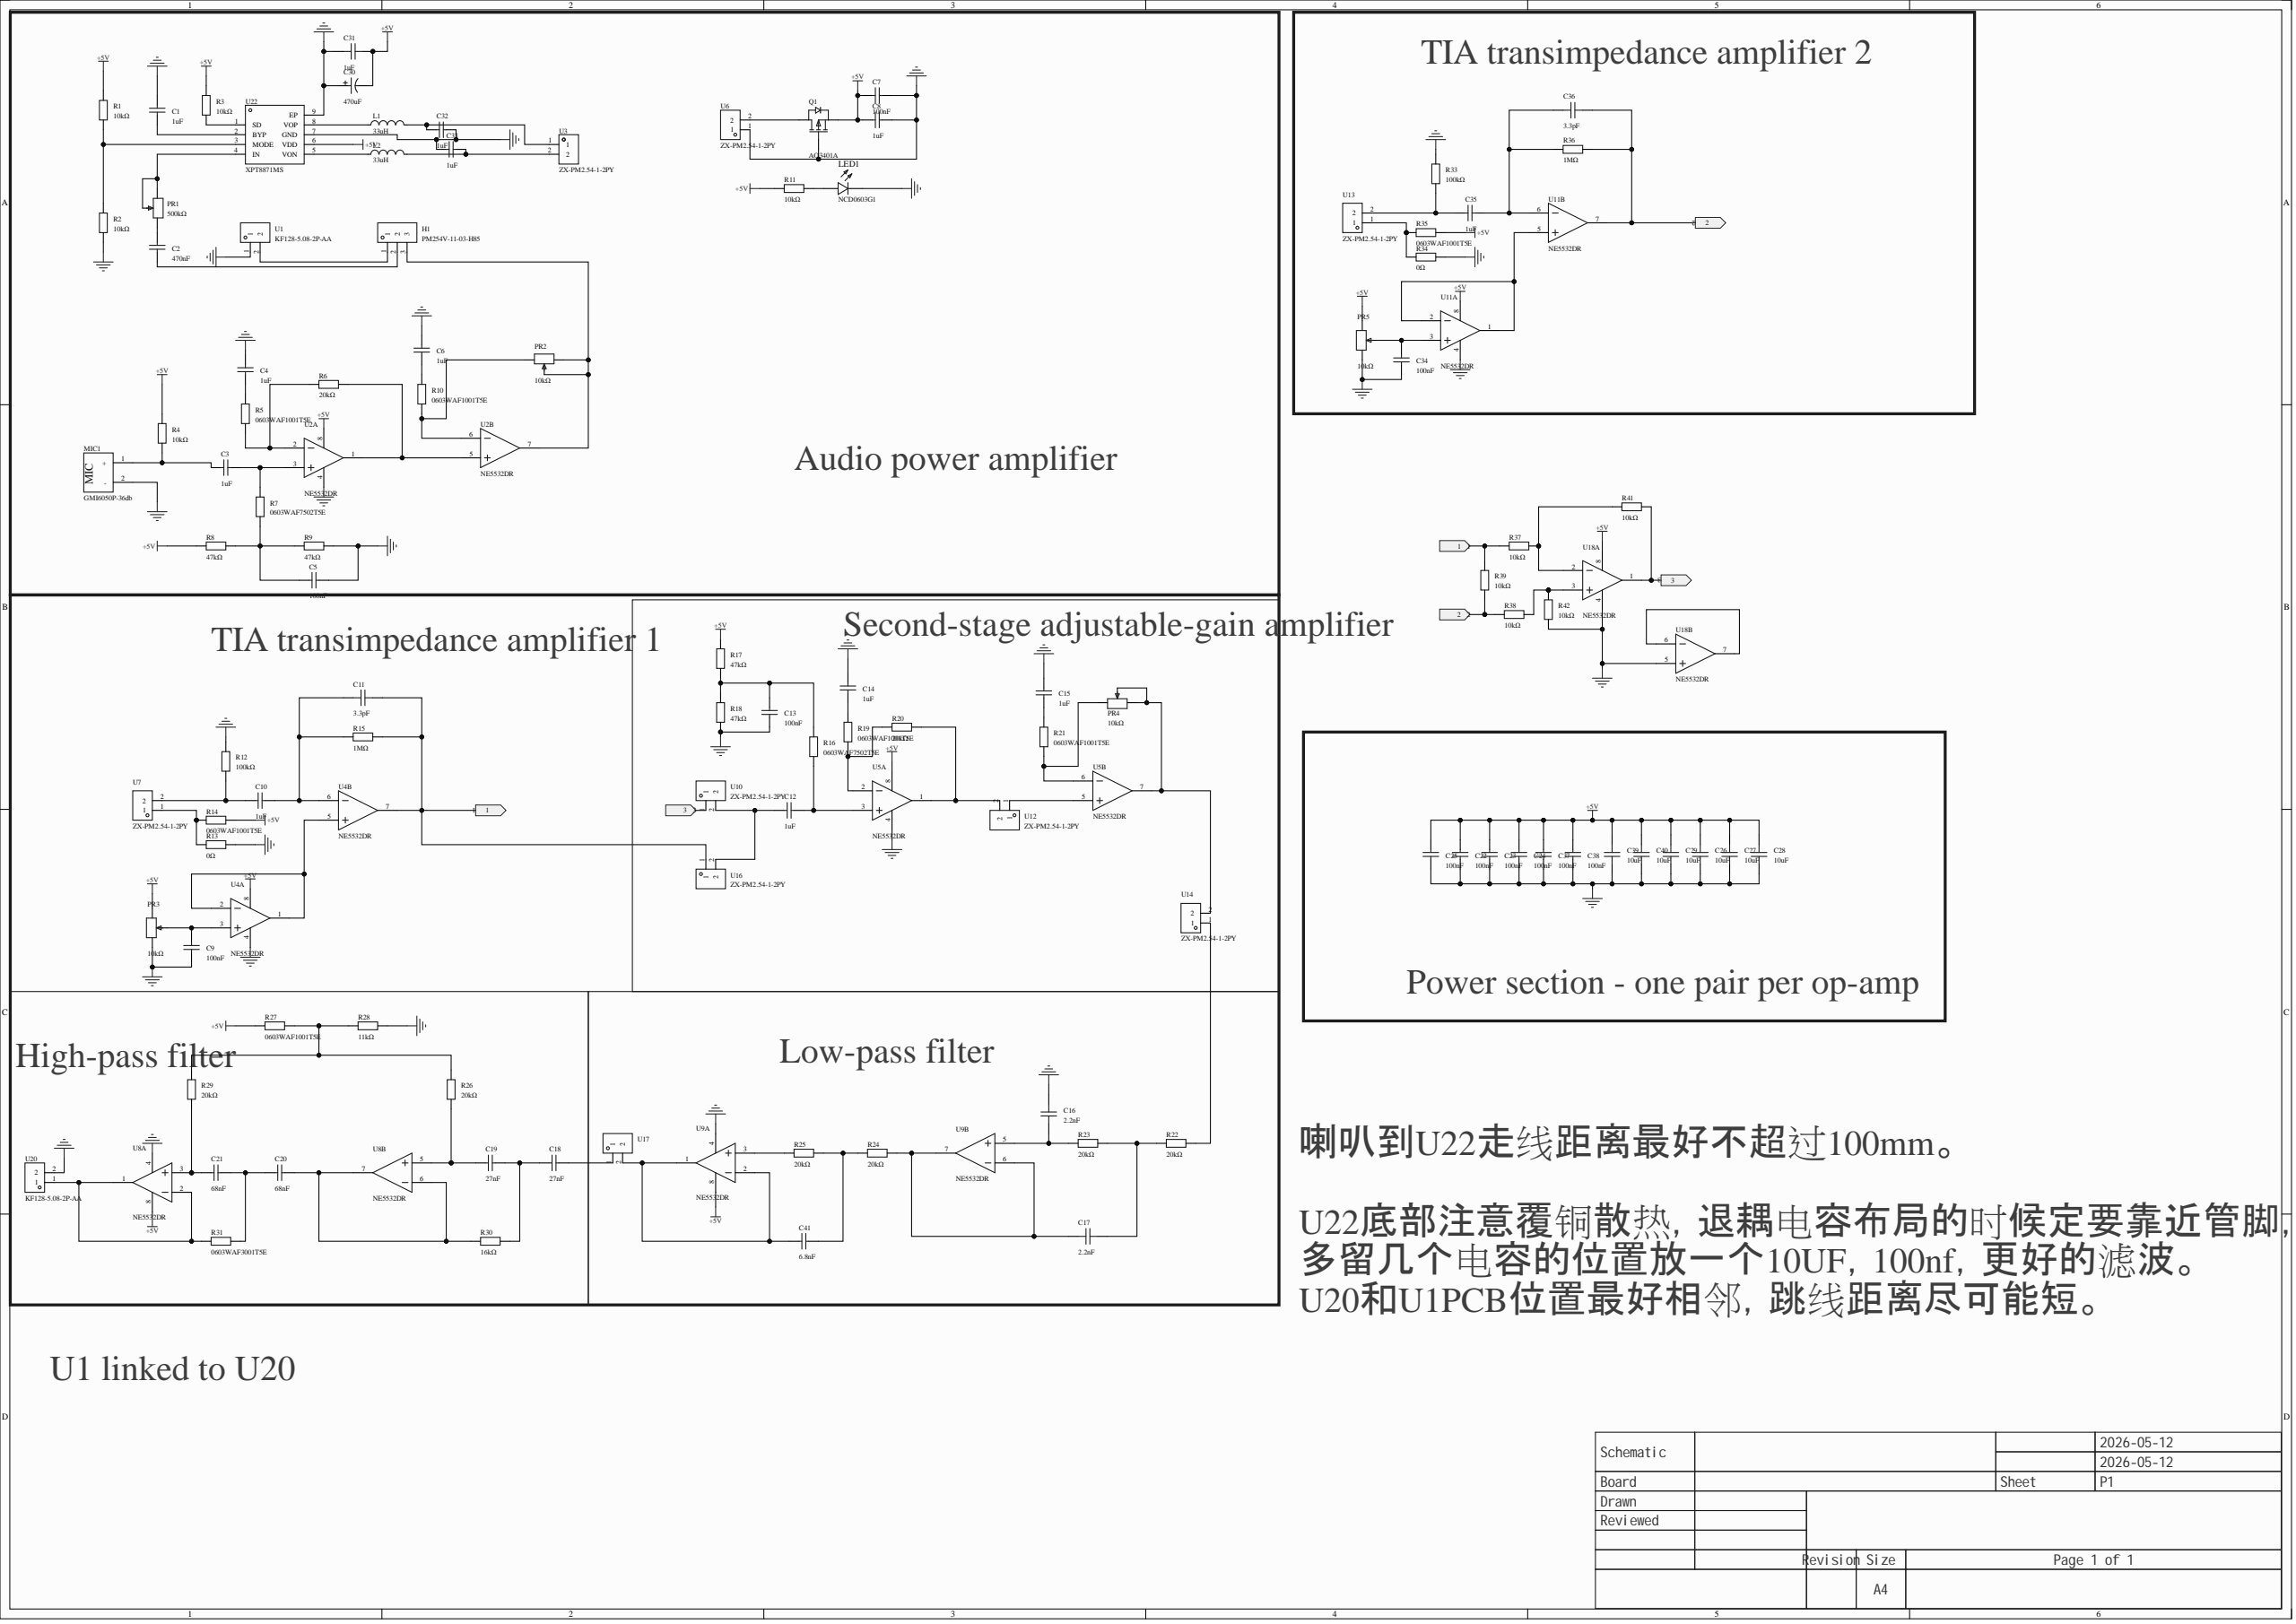Circuit board | Altium Designer | 111 parts | 65 nets
Bill of materials:
Comment,Description,Designator,Footprint,LibRef,Quantity
"1uF","Temperature coefficient: X5R; Tolerance: ±10%; Rated voltage: 50V; Capacitance: 1uF;, Capacitance: 1uF; Tolerance: ±10%; Rated voltage: 50V; Temperature coefficient: X5R;","C1, C3, C4, C6, C8, C10, C12, C14, C15, C31, C32, C33, C35","C0603","CL10A105KB8NNNC","13"
"470nF","Capacitance: 470nF; Tolerance: ±10%; Rated voltage: 16V; Dielectric (temp. coefficient): X7R;","C2","C0603","CC0603KRX7R7BB474","1"
"100nF","Capacitance: 100nF; Tolerance: ±10%; Rated voltage: 100V; Dielectric (temp. coefficient): X7R;","C5, C7, C9, C13, C22, C23, C24, C25, C34, C37, C38","C0805","CC0805KKX7R0BB104","11"
"3.3pF","Capacitance: 3.3pF; Tolerance: ±0.1pF; Rated voltage: 50V; Dielectric (temp. coefficient): NP0;","C11, C36","C0402","CC0402BRNPO9BN3R3","2"
"2.2nF","Temperature coefficient: X7R; Capacitance: 2.2nF; Tolerance: ±10%; Rated voltage: 50V;","C16, C17","C0805","TCC0805X7R222K500DTS","2"
"27nF","Capacitance: 27nF; Tolerance: ±10%; Rated voltage: 50V; Dielectric (temp. coefficient): X7R;","C18, C19","C0603","CC0603KRX7R9BB273","2"
"68nF","Temperature coefficient: X7R; Tolerance: ±10%; Capacitance: 68nF; Rated voltage: 50V;","C20, C21","C0603","CL10B683KB8NNNC","2"
"10uF","Capacitance: 10uF; Tolerance: ±20%; Rated voltage: 25V; Temperature coefficient: X5R;","C26, C27, C28, C29, C39, C40","C0603","CL10A106MA8NRNC","6"
"470uF","Capacitance: 470uF; Tolerance: ±20%; Rated voltage: 35V;","C30","CAP-TH_BD10.0-P5.00-D1.0-FD","35YXJ470M10x16","1"
"6.8nF","Capacitance: 6.8nF; Tolerance: ±10%; Rated voltage: 50V; Dielectric (temp. coefficient): X7R;","C41","C0603","CC0603KRX7R9BB682","1"
"PM254V-11-03-H85","Socket structure: 1x3P; Pitch: 2.54mm; Row spacing: -; Round/square hole: Square; Mounting type: Through-hole; Rows: Single row; Total positions: 3P; Rated current: 3A; Socket orientation: Top; Plastic height: 8.5mm; Contact material: Brass; Contact plating: -; Operating temperature: -40℃~+105℃;","H1","HDR-TH_3P-P2.54-V-F","PM254V-11-03-H85","1"
"33uH","Inductance: 33uH; Tolerance: ±20%; Rated current: 2A; DC resistance (DCR): 270mΩ;","L1, L2","IND-SMD_L7.3-W6.6","MHCI06030-330M-R8","2"
"NCD0603G1","Emitted color: Emerald green;","LED1","LED0603-RD","NCD0603G1","1"
"GMI6050P-36db","","MIC1","MIC-TH_BD6.0-P1.90-D0.4-L-FD_GMI6050P-2CXXDB","GMI6050P-36db","1"
"500kΩ","Resistance: 500kΩ; Tolerance: ±10%; Temperature coefficient: ±100ppm/?;","PR1","RES-ADJ-TH_3296W","3296W-1-504LF","1"
"10kΩ","Resistance: 10kΩ; Tolerance: ±10%; Temperature coefficient: ±100ppm/?;","PR2, PR3, PR4, PR5","RES-ADJ-TH_3296W","3296W-1-103LF","4"
"AO3401A","","Q1","SOT-23_L2.9-W1.3-P1.90-LS2.4-BR","AO3401A_C15127","1"
"10kΩ","","R1, R2, R3, R4, R11, R37, R38, R39, R41, R42","R0603","0603WAF1002T5E","10"
"0603WAF1001T5E","","R5, R10, R14, R19, R21, R27, R35","R0603","0603WAF1001T5E","7"
"20kΩ","","R6, R20, R22, R23, R24, R25, R26, R29","R0603","0603WAF2002T5E","8"
"0603WAF7502T5E","","R7, R16","R0603","0603WAF7502T5E","2"
"47kΩ","","R8, R9, R17, R18","R0603","0603WAF4702T5E","4"
"100kΩ","","R12, R33","R0603","0603WAF1003T5E","2"
"0Ω","","R13, R34","R0603","0603WAF0000T5E","2"
"1MΩ","","R15, R36","R0603","0603WAF1004T5E","2"
"11kΩ","","R28","R0603","0603WAF1102T5E","1"
"16kΩ","","R30","R0603","0603WAF1602T5E","1"
"0603WAF3001T5E","","R31","R0603","0603WAF3001T5E","1"
"KF128-5.08-2P-AA","Structure: 1x2P; Pitch: 5.08mm; Color: Green; Mounting type: Through-hole; Rows: 1; Pins per row: 2; Rated current: 24A; Rated voltage: 250V; Wire gauge - AWG: 12~22; Wire gauge - sq mm: 2.5; Operating temperature: -40℃~+105℃;","U1, U20","CONN-TH_P5.08_KF128-5.08-2P","KF128-5.08-2P-AA","2"
"NE5532DR","Op-amp type: General Purpose; Amplifiers per package: 2; Gain bandwidth product (GBP): 10MHz; Slew rate (SR): 9 V/us; Supply voltage: ±5V ~ 15V; Supply current per channel: 8mA;","U2, U4, U5, U8, U9, U11, U18","SOIC-8_L4.9-W3.9-P1.27-LS6.0-BL","NE5532DR","7"
"ZX-PM2.54-1-2PY","Socket structure: 1x2P; Pitch: 2.54mm; Row spacing: -; Round/square hole: Square; Mounting type: Through-hole; Rows: Single row; Total positions: 2P; Rated current: 3A; Rated voltage: -; Socket orientation: Top; Plastic height: 8.5mm; Contact material: Brass; Contact plating: Gold; Operating temperature: -40℃~+105℃;","U3, U6, U7, U10, U12, U13, U14, U16, U17","HDR-TH_2P-P2.54-V-F","ZX-PM2.54-1-2PY","9"
"XPT8871MS","","U22","ESOP-8_L4.9-W3.9-P1.27-LS6.0-BL-EP","XPT8871MS","1"
Netlist (Protel format):
[
C1
C0603
1uF



]
[
C2
C0603
470nF



]
[
C3
C0603
1uF



]
[
C4
C0603
1uF



]
[
C5
C0805
100nF



]
[
C6
C0603
1uF



]
[
C7
C0805
100nF



]
[
C8
C0603
1uF



]
[
C9
C0805
100nF



]
[
C10
C0603
1uF



]
[
C11
C0402
3.3pF



]
[
C12
C0603
1uF



]
[
C13
C0805
100nF



]
[
C14
C0603
1uF



]
[
C15
C0603
1uF



]
[
C16
C0805
2.2nF



]
[
C17
C0805
2.2nF



]
[
C18
C0603
27nF



]
[
C19
C0603
27nF



]
[
C20
C0603
68nF



]
[
C21
C0603
68nF



]
[
C22
C0805
100nF



]
[
C23
C0805
100nF



]
[
C24
C0805
100nF



]
[
C25
C0805
100nF



]
[
C26
C0603
10uF



]
[
C27
C0603
10uF



]
[
C28
C0603
10uF



]
[
C29
C0603
10uF



]
[
C30
CAP-TH_BD10.0-P5.00-D1.0-FD
470uF



]
[
C31
C0603
1uF



]
[
C32
C0603
1uF



]
[
C33
C0603
1uF



]
[
C34
C0805
100nF



]
[
C35
C0603
1uF



]
[
C36
C0402
3.3pF



]
[
C37
C0805
100nF



]
[
C38
C0805
100nF



]
[
C39
C0603
10uF



]
[
C40
C0603
10uF



]
[
C41
C0603
6.8nF



]
[
H1
HDR-TH_3P-P2.54-V-F
PM254V-11-03-H85



]
[
L1
IND-SMD_L7.3-W6.6
33uH



]
[
L2
IND-SMD_L7.3-W6.6
33uH



]
[
LED1
LED0603-RD
NCD0603G1



]
[
MIC1
MIC-TH_BD6.0-P1.90-D0.4-L-FD_GMI6050P-2CXXDB
GMI6050P-36db



]
[
PR1
RES-ADJ-TH_3296W
500kΩ



]
[
PR2
RES-ADJ-TH_3296W
10kΩ



]
[
PR3
RES-ADJ-TH_3296W
10kΩ



]
[
PR4
RES-ADJ-TH_3296W
10kΩ



]
[
PR5
RES-ADJ-TH_3296W
10kΩ



]
[
Q1
SOT-23_L2.9-W1.3-P1.90-LS2.4-BR
AO3401A



]
[
R1
R0603
10kΩ



]
[
R2
R0603
10kΩ



]
[
R3
R0603
10kΩ



]
[
R4
R0603
10kΩ



]
[
R5
R0603
0603WAF1001T5E



]
[
R6
R0603
20kΩ



]
[
R7
R0603
0603WAF7502T5E



]
[
R8
R0603
47kΩ



]
[
R9
R0603
47kΩ



]
[
R10
R0603
0603WAF1001T5E



]
[
R11
R0603
10kΩ



]
[
R12
R0603
100kΩ



]
[
R13
R0603
0Ω



]
[
R14
R0603
0603WAF1001T5E



]
[
R15
R0603
1MΩ



]
[
R16
R0603
0603WAF7502T5E



]
[
R17
R0603
47kΩ



]
[
R18
R0603
47kΩ



]
[
R19
R0603
0603WAF1001T5E



]
[
R20
R0603
20kΩ



]
[
R21
R0603
0603WAF1001T5E



]
[
R22
R0603
20kΩ



]
[
R23
R0603
20kΩ



]
[
R24
R0603
20kΩ



]
[
R25
R0603
20kΩ



]
[
R26
R0603
20kΩ



]
[
R27
R0603
0603WAF1001T5E



]
[
R28
R0603
11kΩ



]
[
R29
R0603
20kΩ



]
[
R30
R0603
16kΩ



]
[
R31
R0603
0603WAF3001T5E



]
[
R33
R0603
100kΩ



]
[
R34
R0603
0Ω



]
[
R35
R0603
0603WAF1001T5E



]
[
R36
R0603
1MΩ



]
[
R37
R0603
10kΩ



]
[
R38
R0603
10kΩ



]
[
R39
R0603
10kΩ



]
[
R41
R0603
10kΩ



]
[
R42
R0603
10kΩ



]
[
U1
CONN-TH_P5.08_KF128-5.08-2P
KF128-5.08-2P-AA



]
[
U2
SOIC-8_L4.9-W3.9-P1.27-LS6.0-BL
NE5532DR



]
[
U3
HDR-TH_2P-P2.54-V-F
ZX-PM2.54-1-2PY



]
[
U4
SOIC-8_L4.9-W3.9-P1.27-LS6.0-BL
NE5532DR



]
[
U5
SOIC-8_L4.9-W3.9-P1.27-LS6.0-BL
NE5532DR



]
[
U6
HDR-TH_2P-P2.54-V-F
ZX-PM2.54-1-2PY



]
[
U7
HDR-TH_2P-P2.54-V-F
ZX-PM2.54-1-2PY



]
[
U8
SOIC-8_L4.9-W3.9-P1.27-LS6.0-BL
NE5532DR



]
[
U9
SOIC-8_L4.9-W3.9-P1.27-LS6.0-BL
NE5532DR



]
[
U10
HDR-TH_2P-P2.54-V-F
ZX-PM2.54-1-2PY



]
[
U11
SOIC-8_L4.9-W3.9-P1.27-LS6.0-BL
NE5532DR



]
[
U12
HDR-TH_2P-P2.54-V-F
ZX-PM2.54-1-2PY



]
[
U13
HDR-TH_2P-P2.54-V-F
ZX-PM2.54-1-2PY



]
[
U14
HDR-TH_2P-P2.54-V-F
ZX-PM2.54-1-2PY



]
[
U16
HDR-TH_2P-P2.54-V-F
ZX-PM2.54-1-2PY



]
[
U17
HDR-TH_2P-P2.54-V-F
ZX-PM2.54-1-2PY



]
[
U18
SOIC-8_L4.9-W3.9-P1.27-LS6.0-BL
NE5532DR



]
[
U20
CONN-TH_P5.08_KF128-5.08-2P
KF128-5.08-2P-AA



]
[
U22
ESOP-8_L4.9-W3.9-P1.27-LS6.0-BL-EP
XPT8871MS



]
(
NetU18_6
U18-6
U18-7
)
(
NetU11_1
U11-1
U11-2
U11-5
)
(
NetU5_5
U5-5
U12-1
)
(
NetU4_1
U4-1
U4-2
U4-5
)
(
NetR38_2
R38-2
R42-2
U18-3
)
(
NetR37_2
R37-2
R41-2
U18-2
)
(
NetR34_1
R34-1
R35-1
U13-1
)
(
NetR31_1
R31-1
U8-1
U8-2
U20-1
)
(
NetR26_2
R26-2
R27-1
R28-2
R29-1
)
(
NetR25_1
R25-1
U9-3
)
(
NetR22_2
R22-2
U14-1
)
(
NetR20_2
R20-2
U5-1
U12-2
)
(
NetR19_1
R19-1
R20-1
U5-2
)
(
NetR13_1
R13-1
R14-1
U7-1
)
(
NetR6_1
R6-1
U2-1
U2-5
)
(
NetR5_1
R5-1
R6-2
U2-2
)
(
NetR3_1
R3-1
U22-1
)
(
NetR1_1
R1-1
R2-2
U22-3
)
(
NetQ1_3
Q1-3
U6-2
)
(
NetPR4_3
PR4-3
R21-1
U5-6
)
(
NetPR4_1
PR4-1
PR4-2
U5-7
U14-2
)
(
NetPR2_1
PR2-1
R10-2
U2-6
)
(
NetPR1_1
PR1-1
PR1-2
U22-4
)
(
NetLED1_2
LED1-2
R11-2
)
(
NetL2_1
L2-1
U22-5
)
(
NetL1_1
L1-1
U22-8
)
(
NetH1_3
H1-3
PR2-2
PR2-3
U2-7
)
(
NetH1_1
H1-1
U1-2
)
(
NetC41_2
C41-2
R24-1
R25-2
)
(
NetC41_1
C41-1
U9-1
U9-2
U17-2
)
(
NetC35_2
C35-2
C36-2
R36-1
U11-6
)
(
NetC35_1
C35-1
R33-1
U13-2
)
(
NetC34_2
C34-2
PR5-2
U11-3
)
(
NetC33_2
C33-2
L2-2
U3-2
)
(
NetC32_1
C32-1
L1-2
U3-1
)
(
NetC21_1
C21-1
R29-2
U8-3
)
(
NetC20_2
C20-2
R30-1
U8-6
U8-7
)
(
NetC20_1
C20-1
C21-2
R31-2
)
(
NetC19_1
C19-1
R26-1
U8-5
)
(
NetC18_2
C18-2
U17-1
)
(
NetC18_1
C18-1
C19-2
R30-2
)
(
NetC17_2
C17-2
R24-2
U9-6
U9-7
)
(
NetC17_1
C17-1
R22-1
R23-2
)
(
NetC16_2
C16-2
R23-1
U9-5
)
(
NetC15_1
C15-1
R21-2
)
(
NetC14_1
C14-1
R19-2
)
(
NetC13_2
C13-2
R16-2
R17-1
R18-2
)
(
NetC12_2
C12-2
R16-1
U5-3
)
(
NetC12_1
C12-1
U10-2
U16-2
)
(
NetC10_2
C10-2
C11-2
R15-1
U4-6
)
(
NetC10_1
C10-1
R12-1
U7-2
)
(
NetC9_2
C9-2
PR3-2
U4-3
)
(
NetC6_1
C6-1
R10-1
)
(
NetC5_1
C5-1
R7-1
R8-1
R9-2
)
(
NetC4_1
C4-1
R5-2
)
(
NetC3_2
C3-2
R7-2
U2-3
)
(
NetC3_1
C3-1
MIC1-1
R4-1
)
(
NetC2_2
C2-2
PR1-3
)
(
NetC2_1
C2-1
H1-2
)
(
NetC1_1
C1-1
U22-2
)
(
GND
C1-2
C4-2
C5-2
C6-2
C7-2
C8-2
C9-1
C13-1
C14-2
C15-2
C16-1
C22-1
C23-1
C24-1
C25-1
C26-1
C27-1
C28-1
C29-1
C30-1
C31-1
C32-2
C33-1
C34-1
C37-1
C38-1
C39-1
C40-1
LED1-1
MIC1-2
PR3-1
PR5-1
Q1-1
R2-1
R9-1
R12-2
R13-2
R18-1
R28-1
R33-2
R34-2
R42-1
U1-1
U2-4
U4-4
U5-4
U6-1
U8-4
U9-4
U11-4
U18-4
U18-5
U20-2
U22-7
U22-9
)
(
+5V
C7-1
C8-1
C22-2
C23-2
C24-2
C25-2
C26-2
C27-2
C28-2
C29-2
C30-2
C31-2
C37-2
C38-2
C39-2
C40-2
PR3-3
PR5-3
Q1-2
R1-2
R3-2
R4-2
R8-2
R11-1
R14-2
R17-2
R27-2
R35-2
U2-8
U4-8
U5-8
U8-8
U9-8
U11-8
U18-8
U22-6
)
(
3
R41-1
U10-1
U18-1
)
(
2
C36-1
R36-2
R38-1
R39-1
U11-7
)
(
1
C11-1
R15-2
R37-1
R39-2
U4-7
U16-1
)